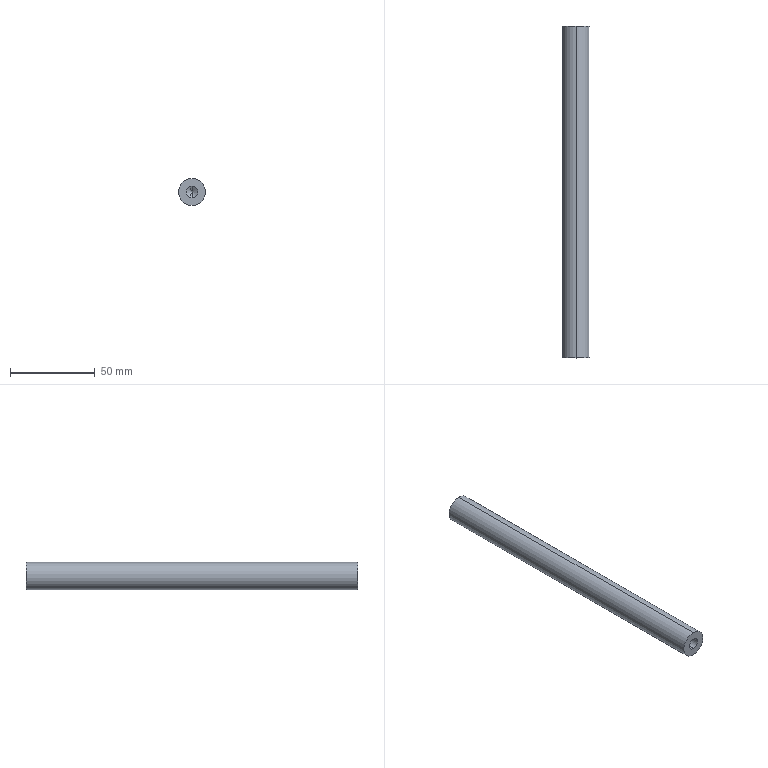Part | SolidWorks | features HoleWzd 2, RevolutionThin 1 | 1 solid | 12 faces | box 16 x 196 x 16 mm | volume 38778 mm3 | cylinder 6 | cone 4 | plane 2 | commonest cylinder face diameters 6.8 x4 16 x2
STEP:
#1=CARTESIAN_POINT('',(0.,188.,-3.4));
#2=VERTEX_POINT('',#1);
#3=CARTESIAN_POINT('',(0.,188.,3.4));
#4=VERTEX_POINT('',#3);
#5=CARTESIAN_POINT('',(0.,188.,0.));
#6=DIRECTION('',(0.,1.,0.));
#7=DIRECTION('',(0.,0.,1.));
#8=AXIS2_PLACEMENT_3D('',#5,#6,#7);
#9=CIRCLE('',#8,3.4);
#10=EDGE_CURVE('',#2,#4,#9,.T.);
#11=ORIENTED_EDGE('',*,*,#10,.F.);
#12=CARTESIAN_POINT('',(0.,196.,-3.4));
#13=VERTEX_POINT('',#12);
#14=CARTESIAN_POINT('',(0.,196.,-3.4));
#15=DIRECTION('',(0.,1.,0.));
#16=VECTOR('',#15,1000.);
#17=LINE('',#14,#16);
#18=EDGE_CURVE('',#2,#13,#17,.T.);
#19=ORIENTED_EDGE('',*,*,#18,.T.);
#20=CARTESIAN_POINT('',(0.,196.,3.4));
#21=VERTEX_POINT('',#20);
#22=CARTESIAN_POINT('',(0.,196.,0.));
#23=DIRECTION('',(0.,1.,0.));
#24=DIRECTION('',(0.,0.,1.));
#25=AXIS2_PLACEMENT_3D('',#22,#23,#24);
#26=CIRCLE('',#25,3.4);
#27=EDGE_CURVE('',#13,#21,#26,.T.);
#28=ORIENTED_EDGE('',*,*,#27,.T.);
#29=CARTESIAN_POINT('',(0.,196.,3.4));
#30=DIRECTION('',(0.,1.,0.));
#31=VECTOR('',#30,1000.);
#32=LINE('',#29,#31);
#33=EDGE_CURVE('',#4,#21,#32,.T.);
#34=ORIENTED_EDGE('',*,*,#33,.F.);
#35=EDGE_LOOP('',(#11,#19,#28,#34));
#36=FACE_OUTER_BOUND('',#35,.T.);
#37=CARTESIAN_POINT('',(0.,196.,0.));
#38=DIRECTION('',(0.,1.,0.));
#39=DIRECTION('',(0.,0.,1.));
#40=AXIS2_PLACEMENT_3D('',#37,#38,#39);
#41=CYLINDRICAL_SURFACE('',#40,3.4);
#42=ADVANCED_FACE('',(#36),#41,.F.);
#43=CARTESIAN_POINT('',(0.,185.957,0.));
#44=VERTEX_POINT('',#43);
#45=CARTESIAN_POINT('',(0.,188.,3.4));
#46=DIRECTION('',(0.,0.515,0.8572));
#47=VECTOR('',#46,1000.);
#48=LINE('',#45,#47);
#49=EDGE_CURVE('',#44,#4,#48,.T.);
#50=ORIENTED_EDGE('',*,*,#49,.F.);
#51=CARTESIAN_POINT('',(0.,188.,-3.4));
#52=DIRECTION('',(0.,0.515,-0.8572));
#53=VECTOR('',#52,1000.);
#54=LINE('',#51,#53);
#55=EDGE_CURVE('',#44,#2,#54,.T.);
#56=ORIENTED_EDGE('',*,*,#55,.T.);
#57=ORIENTED_EDGE('',*,*,#10,.T.);
#58=EDGE_LOOP('',(#50,#56,#57));
#59=FACE_OUTER_BOUND('',#58,.T.);
#60=CARTESIAN_POINT('',(0.,188.,0.));
#61=DIRECTION('',(0.,1.,0.));
#62=DIRECTION('',(0.,0.,1.));
#63=AXIS2_PLACEMENT_3D('',#60,#61,#62);
#64=CONICAL_SURFACE('',#63,3.4,1.03);
#65=ADVANCED_FACE('',(#59),#64,.F.);
#66=CARTESIAN_POINT('',(0.,8.,3.4));
#67=VERTEX_POINT('',#66);
#68=CARTESIAN_POINT('',(0.,8.,-3.4));
#69=VERTEX_POINT('',#68);
#70=CARTESIAN_POINT('',(0.,8.,0.));
#71=DIRECTION('',(0.,-1.,0.));
#72=DIRECTION('',(0.,0.,-1.));
#73=AXIS2_PLACEMENT_3D('',#70,#71,#72);
#74=CIRCLE('',#73,3.4);
#75=EDGE_CURVE('',#67,#69,#74,.T.);
#76=ORIENTED_EDGE('',*,*,#75,.F.);
#77=CARTESIAN_POINT('',(0.,0.,3.4));
#78=VERTEX_POINT('',#77);
#79=CARTESIAN_POINT('',(0.,0.,3.4));
#80=DIRECTION('',(0.,-1.,0.));
#81=VECTOR('',#80,1000.);
#82=LINE('',#79,#81);
#83=EDGE_CURVE('',#67,#78,#82,.T.);
#84=ORIENTED_EDGE('',*,*,#83,.T.);
#85=CARTESIAN_POINT('',(0.,0.,-3.4));
#86=VERTEX_POINT('',#85);
#87=CARTESIAN_POINT('',(0.,0.,0.));
#88=DIRECTION('',(0.,-1.,0.));
#89=DIRECTION('',(0.,0.,-1.));
#90=AXIS2_PLACEMENT_3D('',#87,#88,#89);
#91=CIRCLE('',#90,3.4);
#92=EDGE_CURVE('',#78,#86,#91,.T.);
#93=ORIENTED_EDGE('',*,*,#92,.T.);
#94=CARTESIAN_POINT('',(0.,0.,-3.4));
#95=DIRECTION('',(0.,-1.,0.));
#96=VECTOR('',#95,1000.);
#97=LINE('',#94,#96);
#98=EDGE_CURVE('',#69,#86,#97,.T.);
#99=ORIENTED_EDGE('',*,*,#98,.F.);
#100=EDGE_LOOP('',(#76,#84,#93,#99));
#101=FACE_OUTER_BOUND('',#100,.T.);
#102=CARTESIAN_POINT('',(0.,0.,0.));
#103=DIRECTION('',(0.,-1.,0.));
#104=DIRECTION('',(0.,0.,-1.));
#105=AXIS2_PLACEMENT_3D('',#102,#103,#104);
#106=CYLINDRICAL_SURFACE('',#105,3.4);
#107=ADVANCED_FACE('',(#101),#106,.F.);
#108=CARTESIAN_POINT('',(0.,10.043,0.));
#109=VERTEX_POINT('',#108);
#110=CARTESIAN_POINT('',(0.,8.,-3.4));
#111=DIRECTION('',(0.,-0.515,-0.8572));
#112=VECTOR('',#111,1000.);
#113=LINE('',#110,#112);
#114=EDGE_CURVE('',#109,#69,#113,.T.);
#115=ORIENTED_EDGE('',*,*,#114,.F.);
#116=CARTESIAN_POINT('',(0.,8.,3.4));
#117=DIRECTION('',(0.,-0.515,0.8572));
#118=VECTOR('',#117,1000.);
#119=LINE('',#116,#118);
#120=EDGE_CURVE('',#109,#67,#119,.T.);
#121=ORIENTED_EDGE('',*,*,#120,.T.);
#122=ORIENTED_EDGE('',*,*,#75,.T.);
#123=EDGE_LOOP('',(#115,#121,#122));
#124=FACE_OUTER_BOUND('',#123,.T.);
#125=CARTESIAN_POINT('',(0.,8.,0.));
#126=DIRECTION('',(0.,-1.,0.));
#127=DIRECTION('',(0.,0.,-1.));
#128=AXIS2_PLACEMENT_3D('',#125,#126,#127);
#129=CONICAL_SURFACE('',#128,3.4,1.03);
#130=ADVANCED_FACE('',(#124),#129,.F.);
#131=CARTESIAN_POINT('',(0.,196.,-8.));
#132=VERTEX_POINT('',#131);
#133=CARTESIAN_POINT('',(0.,196.,8.));
#134=VERTEX_POINT('',#133);
#135=CARTESIAN_POINT('',(0.,196.,0.));
#136=DIRECTION('',(0.,-1.,0.));
#137=DIRECTION('',(0.,0.,-1.));
#138=AXIS2_PLACEMENT_3D('',#135,#136,#137);
#139=CIRCLE('',#138,8.);
#140=EDGE_CURVE('',#132,#134,#139,.T.);
#141=ORIENTED_EDGE('',*,*,#140,.T.);
#142=CARTESIAN_POINT('',(0.,0.,8.));
#143=VERTEX_POINT('',#142);
#144=CARTESIAN_POINT('',(0.,0.,8.));
#145=DIRECTION('',(0.,-1.,0.));
#146=VECTOR('',#145,1000.);
#147=LINE('',#144,#146);
#148=EDGE_CURVE('',#134,#143,#147,.T.);
#149=ORIENTED_EDGE('',*,*,#148,.T.);
#150=CARTESIAN_POINT('',(0.,0.,-8.));
#151=VERTEX_POINT('',#150);
#152=CARTESIAN_POINT('',(0.,0.,0.));
#153=DIRECTION('',(0.,-1.,0.));
#154=DIRECTION('',(0.,0.,-1.));
#155=AXIS2_PLACEMENT_3D('',#152,#153,#154);
#156=CIRCLE('',#155,8.);
#157=EDGE_CURVE('',#151,#143,#156,.T.);
#158=ORIENTED_EDGE('',*,*,#157,.F.);
#159=CARTESIAN_POINT('',(0.,0.,-8.));
#160=DIRECTION('',(0.,-1.,0.));
#161=VECTOR('',#160,1000.);
#162=LINE('',#159,#161);
#163=EDGE_CURVE('',#132,#151,#162,.T.);
#164=ORIENTED_EDGE('',*,*,#163,.F.);
#165=EDGE_LOOP('',(#141,#149,#158,#164));
#166=FACE_OUTER_BOUND('',#165,.T.);
#167=CARTESIAN_POINT('',(0.,0.,0.));
#168=DIRECTION('',(0.,-1.,0.));
#169=DIRECTION('',(0.,0.,-1.));
#170=AXIS2_PLACEMENT_3D('',#167,#168,#169);
#171=CYLINDRICAL_SURFACE('',#170,8.);
#172=ADVANCED_FACE('',(#166),#171,.T.);
#173=ORIENTED_EDGE('',*,*,#148,.F.);
#174=CARTESIAN_POINT('',(0.,196.,0.));
#175=DIRECTION('',(0.,-1.,0.));
#176=DIRECTION('',(0.,0.,-1.));
#177=AXIS2_PLACEMENT_3D('',#174,#175,#176);
#178=CIRCLE('',#177,8.);
#179=EDGE_CURVE('',#134,#132,#178,.T.);
#180=ORIENTED_EDGE('',*,*,#179,.T.);
#181=ORIENTED_EDGE('',*,*,#163,.T.);
#182=CARTESIAN_POINT('',(0.,0.,0.));
#183=DIRECTION('',(0.,-1.,0.));
#184=DIRECTION('',(0.,0.,-1.));
#185=AXIS2_PLACEMENT_3D('',#182,#183,#184);
#186=CIRCLE('',#185,8.);
#187=EDGE_CURVE('',#143,#151,#186,.T.);
#188=ORIENTED_EDGE('',*,*,#187,.F.);
#189=EDGE_LOOP('',(#173,#180,#181,#188));
#190=FACE_OUTER_BOUND('',#189,.T.);
#191=CARTESIAN_POINT('',(0.,0.,0.));
#192=DIRECTION('',(0.,-1.,0.));
#193=DIRECTION('',(0.,0.,-1.));
#194=AXIS2_PLACEMENT_3D('',#191,#192,#193);
#195=CYLINDRICAL_SURFACE('',#194,8.);
#196=ADVANCED_FACE('',(#190),#195,.T.);
#197=CARTESIAN_POINT('',(0.,0.,0.));
#198=DIRECTION('',(0.,-1.,0.));
#199=DIRECTION('',(0.,0.,-1.));
#200=AXIS2_PLACEMENT_3D('',#197,#198,#199);
#201=CIRCLE('',#200,3.4);
#202=EDGE_CURVE('',#86,#78,#201,.T.);
#203=ORIENTED_EDGE('',*,*,#202,.F.);
#204=ORIENTED_EDGE('',*,*,#92,.F.);
#205=EDGE_LOOP('',(#203,#204));
#206=FACE_BOUND('',#205,.T.);
#207=ORIENTED_EDGE('',*,*,#157,.T.);
#208=ORIENTED_EDGE('',*,*,#187,.T.);
#209=EDGE_LOOP('',(#207,#208));
#210=FACE_OUTER_BOUND('',#209,.T.);
#211=CARTESIAN_POINT('',(8.,0.,0.));
#212=DIRECTION('',(0.,1.,0.));
#213=DIRECTION('',(0.,0.,1.));
#214=AXIS2_PLACEMENT_3D('',#211,#212,#213);
#215=PLANE('',#214);
#216=ADVANCED_FACE('',(#206,#210),#215,.F.);
#217=CARTESIAN_POINT('',(0.,196.,0.));
#218=DIRECTION('',(0.,1.,0.));
#219=DIRECTION('',(0.,0.,1.));
#220=AXIS2_PLACEMENT_3D('',#217,#218,#219);
#221=CIRCLE('',#220,3.4);
#222=EDGE_CURVE('',#21,#13,#221,.T.);
#223=ORIENTED_EDGE('',*,*,#222,.F.);
#224=ORIENTED_EDGE('',*,*,#27,.F.);
#225=EDGE_LOOP('',(#223,#224));
#226=FACE_BOUND('',#225,.T.);
#227=ORIENTED_EDGE('',*,*,#140,.F.);
#228=ORIENTED_EDGE('',*,*,#179,.F.);
#229=EDGE_LOOP('',(#227,#228));
#230=FACE_OUTER_BOUND('',#229,.T.);
#231=CARTESIAN_POINT('',(0.,196.,0.));
#232=DIRECTION('',(0.,-1.,0.));
#233=DIRECTION('',(0.,0.,-1.));
#234=AXIS2_PLACEMENT_3D('',#231,#232,#233);
#235=PLANE('',#234);
#236=ADVANCED_FACE('',(#226,#230),#235,.F.);
#237=ORIENTED_EDGE('',*,*,#120,.F.);
#238=ORIENTED_EDGE('',*,*,#114,.T.);
#239=CARTESIAN_POINT('',(0.,8.,0.));
#240=DIRECTION('',(0.,-1.,0.));
#241=DIRECTION('',(0.,0.,-1.));
#242=AXIS2_PLACEMENT_3D('',#239,#240,#241);
#243=CIRCLE('',#242,3.4);
#244=EDGE_CURVE('',#69,#67,#243,.T.);
#245=ORIENTED_EDGE('',*,*,#244,.T.);
#246=EDGE_LOOP('',(#237,#238,#245));
#247=FACE_OUTER_BOUND('',#246,.T.);
#248=CARTESIAN_POINT('',(0.,8.,0.));
#249=DIRECTION('',(0.,-1.,0.));
#250=DIRECTION('',(0.,0.,-1.));
#251=AXIS2_PLACEMENT_3D('',#248,#249,#250);
#252=CONICAL_SURFACE('',#251,3.4,1.03);
#253=ADVANCED_FACE('',(#247),#252,.F.);
#254=ORIENTED_EDGE('',*,*,#83,.F.);
#255=ORIENTED_EDGE('',*,*,#244,.F.);
#256=ORIENTED_EDGE('',*,*,#98,.T.);
#257=ORIENTED_EDGE('',*,*,#202,.T.);
#258=EDGE_LOOP('',(#254,#255,#256,#257));
#259=FACE_OUTER_BOUND('',#258,.T.);
#260=CARTESIAN_POINT('',(0.,0.,0.));
#261=DIRECTION('',(0.,-1.,0.));
#262=DIRECTION('',(0.,0.,-1.));
#263=AXIS2_PLACEMENT_3D('',#260,#261,#262);
#264=CYLINDRICAL_SURFACE('',#263,3.4);
#265=ADVANCED_FACE('',(#259),#264,.F.);
#266=ORIENTED_EDGE('',*,*,#55,.F.);
#267=ORIENTED_EDGE('',*,*,#49,.T.);
#268=CARTESIAN_POINT('',(0.,188.,0.));
#269=DIRECTION('',(0.,1.,0.));
#270=DIRECTION('',(0.,0.,1.));
#271=AXIS2_PLACEMENT_3D('',#268,#269,#270);
#272=CIRCLE('',#271,3.4);
#273=EDGE_CURVE('',#4,#2,#272,.T.);
#274=ORIENTED_EDGE('',*,*,#273,.T.);
#275=EDGE_LOOP('',(#266,#267,#274));
#276=FACE_OUTER_BOUND('',#275,.T.);
#277=CARTESIAN_POINT('',(0.,188.,0.));
#278=DIRECTION('',(0.,1.,0.));
#279=DIRECTION('',(0.,0.,1.));
#280=AXIS2_PLACEMENT_3D('',#277,#278,#279);
#281=CONICAL_SURFACE('',#280,3.4,1.03);
#282=ADVANCED_FACE('',(#276),#281,.F.);
#283=ORIENTED_EDGE('',*,*,#18,.F.);
#284=ORIENTED_EDGE('',*,*,#273,.F.);
#285=ORIENTED_EDGE('',*,*,#33,.T.);
#286=ORIENTED_EDGE('',*,*,#222,.T.);
#287=EDGE_LOOP('',(#283,#284,#285,#286));
#288=FACE_OUTER_BOUND('',#287,.T.);
#289=CARTESIAN_POINT('',(0.,196.,0.));
#290=DIRECTION('',(0.,1.,0.));
#291=DIRECTION('',(0.,0.,1.));
#292=AXIS2_PLACEMENT_3D('',#289,#290,#291);
#293=CYLINDRICAL_SURFACE('',#292,3.4);
#294=ADVANCED_FACE('',(#288),#293,.F.);
#295=CLOSED_SHELL('',(#42,#65,#107,#130,#172,#196,#216,#236,#253,#265,#282,#294));
#296=MANIFOLD_SOLID_BREP('',#295);
#297=CARTESIAN_POINT('',(0.,0.,0.));
#298=DIRECTION('',(0.,0.,1.));
#299=DIRECTION('',(1.,0.,0.));
#300=AXIS2_PLACEMENT_3D('',#297,#298,#299);
#301=(LENGTH_UNIT()NAMED_UNIT(*)SI_UNIT(.MILLI.,.METRE.));
#302=UNCERTAINTY_MEASURE_WITH_UNIT(LENGTH_MEASURE(0.00001),#301,'','');
#303=(NAMED_UNIT(*)PLANE_ANGLE_UNIT()SI_UNIT($,.RADIAN.));
#304=(NAMED_UNIT(*)SI_UNIT($,.STERADIAN.)SOLID_ANGLE_UNIT());
#305=(GEOMETRIC_REPRESENTATION_CONTEXT(3)GLOBAL_UNCERTAINTY_ASSIGNED_CONTEXT((#302))GLOBAL_UNIT_ASSIGNED_CONTEXT((#301,#303,#304))REPRESENTATION_CONTEXT('',''));
#306=ADVANCED_BREP_SHAPE_REPRESENTATION('',(#296,#300),#305);